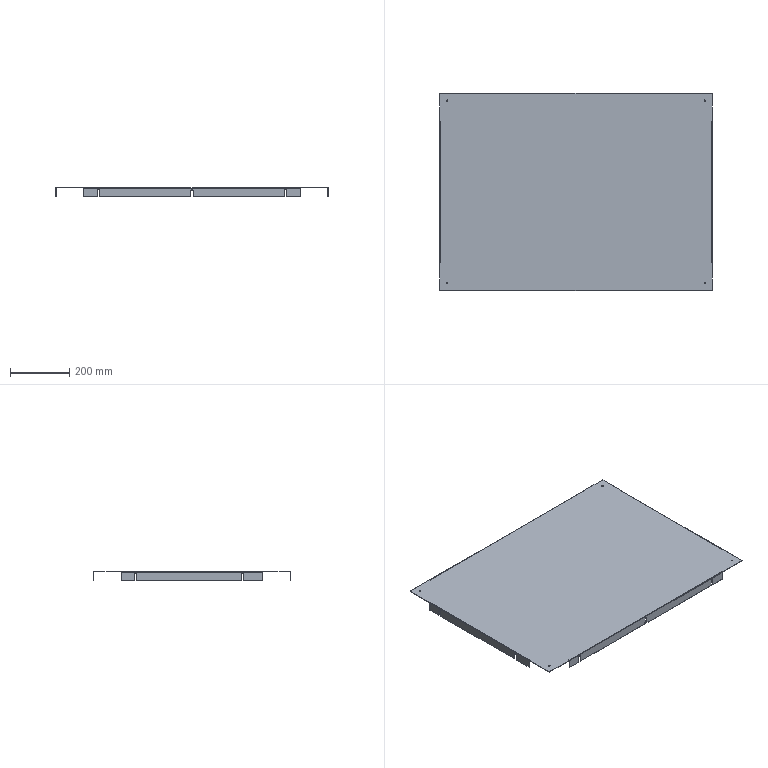Part | STEP file | Front Sheet Metal Cover Plate | 1 solid | 156 faces | box 918 x 665 x 30 mm | volume 1014698 mm3 | plane 92 | cylinder 64 | commonest cylinder face diameters 4 x32 7 x16 4.5 x8 0.2 x4 3.2 x4